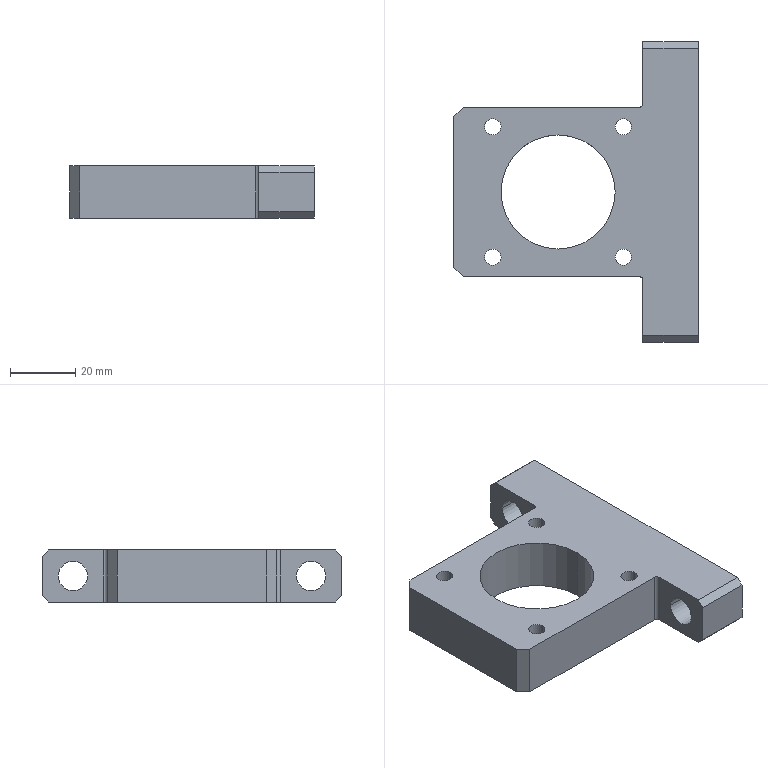Part | STEP file | J454-EBZ05-08-00-Part-1 | 1 solid | 46 faces | box 75 x 92 x 16 mm | volume 52479 mm3 | cylinder 24 | plane 18 | cone 4 | commonest cylinder face diameters 5 x8 7.5 x4 8 x4 9 x4 2 x2 35 x2